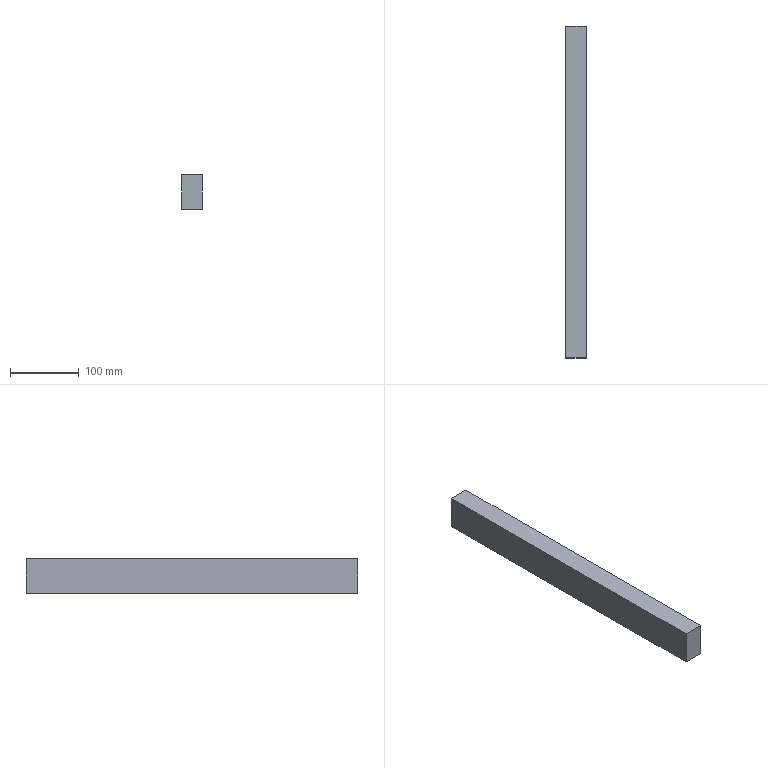Part | SolidWorks | features Extrusion 1 | 1 solid | 6 faces | box 30 x 483.5 x 50 mm | volume 725250 mm3 | plane 6
STEP:
#1=CARTESIAN_POINT('',(15.,-241.75,0.));
#2=VERTEX_POINT('',#1);
#3=CARTESIAN_POINT('',(15.,241.75,0.));
#4=VERTEX_POINT('',#3);
#5=CARTESIAN_POINT('',(15.,241.75,0.));
#6=DIRECTION('',(0.,1.,0.));
#7=VECTOR('',#6,1000.);
#8=LINE('',#5,#7);
#9=EDGE_CURVE('',#2,#4,#8,.T.);
#10=ORIENTED_EDGE('',*,*,#9,.T.);
#11=CARTESIAN_POINT('',(15.,241.75,50.));
#12=VERTEX_POINT('',#11);
#13=CARTESIAN_POINT('',(15.,241.75,50.));
#14=DIRECTION('',(0.,0.,-1.));
#15=VECTOR('',#14,1000.);
#16=LINE('',#13,#15);
#17=EDGE_CURVE('',#12,#4,#16,.T.);
#18=ORIENTED_EDGE('',*,*,#17,.F.);
#19=CARTESIAN_POINT('',(15.,-241.75,50.));
#20=VERTEX_POINT('',#19);
#21=CARTESIAN_POINT('',(15.,241.75,50.));
#22=DIRECTION('',(0.,1.,0.));
#23=VECTOR('',#22,1000.);
#24=LINE('',#21,#23);
#25=EDGE_CURVE('',#20,#12,#24,.T.);
#26=ORIENTED_EDGE('',*,*,#25,.F.);
#27=CARTESIAN_POINT('',(15.,-241.75,50.));
#28=DIRECTION('',(0.,0.,-1.));
#29=VECTOR('',#28,1000.);
#30=LINE('',#27,#29);
#31=EDGE_CURVE('',#20,#2,#30,.T.);
#32=ORIENTED_EDGE('',*,*,#31,.T.);
#33=EDGE_LOOP('',(#10,#18,#26,#32));
#34=FACE_OUTER_BOUND('',#33,.T.);
#35=CARTESIAN_POINT('',(15.,241.75,50.));
#36=DIRECTION('',(-1.,0.,0.));
#37=DIRECTION('',(0.,-1.,0.));
#38=AXIS2_PLACEMENT_3D('',#35,#36,#37);
#39=PLANE('',#38);
#40=ADVANCED_FACE('',(#34),#39,.F.);
#41=CARTESIAN_POINT('',(-15.,241.75,0.));
#42=VERTEX_POINT('',#41);
#43=CARTESIAN_POINT('',(-15.,241.75,0.));
#44=DIRECTION('',(-1.,0.,0.));
#45=VECTOR('',#44,1000.);
#46=LINE('',#43,#45);
#47=EDGE_CURVE('',#4,#42,#46,.T.);
#48=ORIENTED_EDGE('',*,*,#47,.T.);
#49=CARTESIAN_POINT('',(-15.,241.75,50.));
#50=VERTEX_POINT('',#49);
#51=CARTESIAN_POINT('',(-15.,241.75,50.));
#52=DIRECTION('',(0.,0.,-1.));
#53=VECTOR('',#52,1000.);
#54=LINE('',#51,#53);
#55=EDGE_CURVE('',#50,#42,#54,.T.);
#56=ORIENTED_EDGE('',*,*,#55,.F.);
#57=CARTESIAN_POINT('',(-15.,241.75,50.));
#58=DIRECTION('',(-1.,0.,0.));
#59=VECTOR('',#58,1000.);
#60=LINE('',#57,#59);
#61=EDGE_CURVE('',#12,#50,#60,.T.);
#62=ORIENTED_EDGE('',*,*,#61,.F.);
#63=ORIENTED_EDGE('',*,*,#17,.T.);
#64=EDGE_LOOP('',(#48,#56,#62,#63));
#65=FACE_OUTER_BOUND('',#64,.T.);
#66=CARTESIAN_POINT('',(-15.,241.75,50.));
#67=DIRECTION('',(0.,-1.,0.));
#68=DIRECTION('',(0.,0.,-1.));
#69=AXIS2_PLACEMENT_3D('',#66,#67,#68);
#70=PLANE('',#69);
#71=ADVANCED_FACE('',(#65),#70,.F.);
#72=CARTESIAN_POINT('',(-15.,-241.75,0.));
#73=VERTEX_POINT('',#72);
#74=CARTESIAN_POINT('',(-15.,241.75,0.));
#75=DIRECTION('',(0.,-1.,0.));
#76=VECTOR('',#75,1000.);
#77=LINE('',#74,#76);
#78=EDGE_CURVE('',#42,#73,#77,.T.);
#79=ORIENTED_EDGE('',*,*,#78,.T.);
#80=CARTESIAN_POINT('',(-15.,-241.75,50.));
#81=VERTEX_POINT('',#80);
#82=CARTESIAN_POINT('',(-15.,-241.75,50.));
#83=DIRECTION('',(0.,0.,-1.));
#84=VECTOR('',#83,1000.);
#85=LINE('',#82,#84);
#86=EDGE_CURVE('',#81,#73,#85,.T.);
#87=ORIENTED_EDGE('',*,*,#86,.F.);
#88=CARTESIAN_POINT('',(-15.,241.75,50.));
#89=DIRECTION('',(0.,-1.,0.));
#90=VECTOR('',#89,1000.);
#91=LINE('',#88,#90);
#92=EDGE_CURVE('',#50,#81,#91,.T.);
#93=ORIENTED_EDGE('',*,*,#92,.F.);
#94=ORIENTED_EDGE('',*,*,#55,.T.);
#95=EDGE_LOOP('',(#79,#87,#93,#94));
#96=FACE_OUTER_BOUND('',#95,.T.);
#97=CARTESIAN_POINT('',(-15.,241.75,50.));
#98=DIRECTION('',(1.,0.,0.));
#99=DIRECTION('',(0.,1.,0.));
#100=AXIS2_PLACEMENT_3D('',#97,#98,#99);
#101=PLANE('',#100);
#102=ADVANCED_FACE('',(#96),#101,.F.);
#103=CARTESIAN_POINT('',(-15.,-241.75,0.));
#104=DIRECTION('',(1.,0.,0.));
#105=VECTOR('',#104,1000.);
#106=LINE('',#103,#105);
#107=EDGE_CURVE('',#73,#2,#106,.T.);
#108=ORIENTED_EDGE('',*,*,#107,.T.);
#109=ORIENTED_EDGE('',*,*,#31,.F.);
#110=CARTESIAN_POINT('',(-15.,-241.75,50.));
#111=DIRECTION('',(1.,0.,0.));
#112=VECTOR('',#111,1000.);
#113=LINE('',#110,#112);
#114=EDGE_CURVE('',#81,#20,#113,.T.);
#115=ORIENTED_EDGE('',*,*,#114,.F.);
#116=ORIENTED_EDGE('',*,*,#86,.T.);
#117=EDGE_LOOP('',(#108,#109,#115,#116));
#118=FACE_OUTER_BOUND('',#117,.T.);
#119=CARTESIAN_POINT('',(-15.,-241.75,50.));
#120=DIRECTION('',(0.,1.,0.));
#121=DIRECTION('',(0.,0.,1.));
#122=AXIS2_PLACEMENT_3D('',#119,#120,#121);
#123=PLANE('',#122);
#124=ADVANCED_FACE('',(#118),#123,.F.);
#125=ORIENTED_EDGE('',*,*,#25,.T.);
#126=ORIENTED_EDGE('',*,*,#61,.T.);
#127=ORIENTED_EDGE('',*,*,#92,.T.);
#128=ORIENTED_EDGE('',*,*,#114,.T.);
#129=EDGE_LOOP('',(#125,#126,#127,#128));
#130=FACE_OUTER_BOUND('',#129,.T.);
#131=CARTESIAN_POINT('',(0.,0.,50.));
#132=DIRECTION('',(0.,0.,1.));
#133=DIRECTION('',(1.,0.,0.));
#134=AXIS2_PLACEMENT_3D('',#131,#132,#133);
#135=PLANE('',#134);
#136=ADVANCED_FACE('',(#130),#135,.T.);
#137=ORIENTED_EDGE('',*,*,#9,.F.);
#138=ORIENTED_EDGE('',*,*,#107,.F.);
#139=ORIENTED_EDGE('',*,*,#78,.F.);
#140=ORIENTED_EDGE('',*,*,#47,.F.);
#141=EDGE_LOOP('',(#137,#138,#139,#140));
#142=FACE_OUTER_BOUND('',#141,.T.);
#143=CARTESIAN_POINT('',(0.,0.,0.));
#144=DIRECTION('',(0.,0.,1.));
#145=DIRECTION('',(1.,0.,0.));
#146=AXIS2_PLACEMENT_3D('',#143,#144,#145);
#147=PLANE('',#146);
#148=ADVANCED_FACE('',(#142),#147,.F.);
#149=CLOSED_SHELL('',(#40,#71,#102,#124,#136,#148));
#150=MANIFOLD_SOLID_BREP('',#149);
#151=CARTESIAN_POINT('',(0.,0.,0.));
#152=DIRECTION('',(0.,0.,1.));
#153=DIRECTION('',(1.,0.,0.));
#154=AXIS2_PLACEMENT_3D('',#151,#152,#153);
#155=(LENGTH_UNIT()NAMED_UNIT(*)SI_UNIT(.MILLI.,.METRE.));
#156=UNCERTAINTY_MEASURE_WITH_UNIT(LENGTH_MEASURE(0.00001),#155,'','');
#157=(NAMED_UNIT(*)PLANE_ANGLE_UNIT()SI_UNIT($,.RADIAN.));
#158=(NAMED_UNIT(*)SI_UNIT($,.STERADIAN.)SOLID_ANGLE_UNIT());
#159=(GEOMETRIC_REPRESENTATION_CONTEXT(3)GLOBAL_UNCERTAINTY_ASSIGNED_CONTEXT((#156))GLOBAL_UNIT_ASSIGNED_CONTEXT((#155,#157,#158))REPRESENTATION_CONTEXT('',''));
#160=ADVANCED_BREP_SHAPE_REPRESENTATION('',(#150,#154),#159);